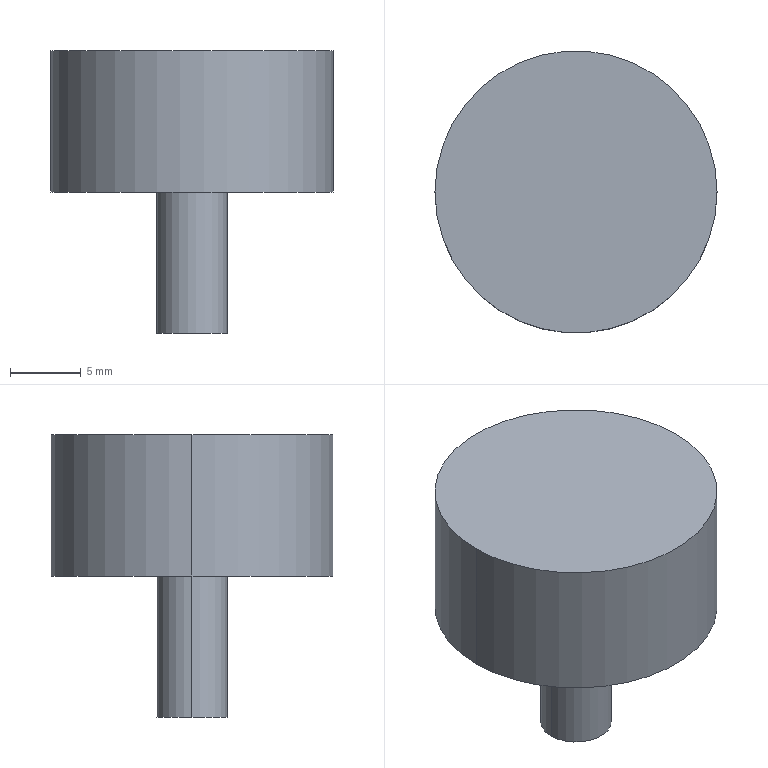Part | SolidWorks | features Extrusion 1, ICE 1 | 1 solid | 7 faces | box 20 x 20 x 20 mm | volume 3338 mm3 | cylinder 4 | plane 3 | commonest cylinder face diameters 5 x2 20 x2
STEP:
#1=CARTESIAN_POINT('',(10.,0.,20.));
#2=VERTEX_POINT('',#1);
#3=CARTESIAN_POINT('',(-10.,0.,20.));
#4=VERTEX_POINT('',#3);
#5=CARTESIAN_POINT('',(0.,0.,20.));
#6=DIRECTION('',(0.,0.,1.));
#7=DIRECTION('',(1.,0.,0.));
#8=AXIS2_PLACEMENT_3D('',#5,#6,#7);
#9=CIRCLE('',#8,10.);
#10=EDGE_CURVE('',#2,#4,#9,.T.);
#11=ORIENTED_EDGE('',*,*,#10,.F.);
#12=CARTESIAN_POINT('',(10.,0.,10.));
#13=VERTEX_POINT('',#12);
#14=CARTESIAN_POINT('',(10.,0.,20.));
#15=DIRECTION('',(0.,0.,-1.));
#16=VECTOR('',#15,1000.);
#17=LINE('',#14,#16);
#18=EDGE_CURVE('',#2,#13,#17,.T.);
#19=ORIENTED_EDGE('',*,*,#18,.T.);
#20=CARTESIAN_POINT('',(-10.,0.,10.));
#21=VERTEX_POINT('',#20);
#22=CARTESIAN_POINT('',(0.,0.,10.));
#23=DIRECTION('',(0.,0.,1.));
#24=DIRECTION('',(1.,0.,0.));
#25=AXIS2_PLACEMENT_3D('',#22,#23,#24);
#26=CIRCLE('',#25,10.);
#27=EDGE_CURVE('',#13,#21,#26,.T.);
#28=ORIENTED_EDGE('',*,*,#27,.T.);
#29=CARTESIAN_POINT('',(-10.,0.,20.));
#30=DIRECTION('',(0.,0.,-1.));
#31=VECTOR('',#30,1000.);
#32=LINE('',#29,#31);
#33=EDGE_CURVE('',#4,#21,#32,.T.);
#34=ORIENTED_EDGE('',*,*,#33,.F.);
#35=EDGE_LOOP('',(#11,#19,#28,#34));
#36=FACE_OUTER_BOUND('',#35,.T.);
#37=CARTESIAN_POINT('',(0.,0.,20.));
#38=DIRECTION('',(0.,0.,-1.));
#39=DIRECTION('',(-1.,0.,0.));
#40=AXIS2_PLACEMENT_3D('',#37,#38,#39);
#41=CYLINDRICAL_SURFACE('',#40,10.);
#42=ADVANCED_FACE('',(#36),#41,.T.);
#43=CARTESIAN_POINT('',(2.5,0.,10.));
#44=VERTEX_POINT('',#43);
#45=CARTESIAN_POINT('',(-2.5,0.,10.));
#46=VERTEX_POINT('',#45);
#47=CARTESIAN_POINT('',(0.,0.,10.));
#48=DIRECTION('',(0.,0.,1.));
#49=DIRECTION('',(1.,0.,0.));
#50=AXIS2_PLACEMENT_3D('',#47,#48,#49);
#51=CIRCLE('',#50,2.5);
#52=EDGE_CURVE('',#44,#46,#51,.T.);
#53=ORIENTED_EDGE('',*,*,#52,.F.);
#54=CARTESIAN_POINT('',(2.5,0.,0.));
#55=VERTEX_POINT('',#54);
#56=CARTESIAN_POINT('',(2.5,0.,10.));
#57=DIRECTION('',(0.,0.,-1.));
#58=VECTOR('',#57,1000.);
#59=LINE('',#56,#58);
#60=EDGE_CURVE('',#44,#55,#59,.T.);
#61=ORIENTED_EDGE('',*,*,#60,.T.);
#62=CARTESIAN_POINT('',(-2.5,0.,0.));
#63=VERTEX_POINT('',#62);
#64=CARTESIAN_POINT('',(0.,0.,0.));
#65=DIRECTION('',(0.,0.,1.));
#66=DIRECTION('',(1.,0.,0.));
#67=AXIS2_PLACEMENT_3D('',#64,#65,#66);
#68=CIRCLE('',#67,2.5);
#69=EDGE_CURVE('',#55,#63,#68,.T.);
#70=ORIENTED_EDGE('',*,*,#69,.T.);
#71=CARTESIAN_POINT('',(-2.5,0.,10.));
#72=DIRECTION('',(0.,0.,-1.));
#73=VECTOR('',#72,1000.);
#74=LINE('',#71,#73);
#75=EDGE_CURVE('',#46,#63,#74,.T.);
#76=ORIENTED_EDGE('',*,*,#75,.F.);
#77=EDGE_LOOP('',(#53,#61,#70,#76));
#78=FACE_OUTER_BOUND('',#77,.T.);
#79=CARTESIAN_POINT('',(0.,0.,10.));
#80=DIRECTION('',(0.,0.,-1.));
#81=DIRECTION('',(-1.,0.,0.));
#82=AXIS2_PLACEMENT_3D('',#79,#80,#81);
#83=CYLINDRICAL_SURFACE('',#82,2.5);
#84=ADVANCED_FACE('',(#78),#83,.T.);
#85=ORIENTED_EDGE('',*,*,#60,.F.);
#86=CARTESIAN_POINT('',(0.,0.,10.));
#87=DIRECTION('',(0.,0.,1.));
#88=DIRECTION('',(1.,0.,0.));
#89=AXIS2_PLACEMENT_3D('',#86,#87,#88);
#90=CIRCLE('',#89,2.5);
#91=EDGE_CURVE('',#46,#44,#90,.T.);
#92=ORIENTED_EDGE('',*,*,#91,.F.);
#93=ORIENTED_EDGE('',*,*,#75,.T.);
#94=CARTESIAN_POINT('',(0.,0.,0.));
#95=DIRECTION('',(0.,0.,1.));
#96=DIRECTION('',(1.,0.,0.));
#97=AXIS2_PLACEMENT_3D('',#94,#95,#96);
#98=CIRCLE('',#97,2.5);
#99=EDGE_CURVE('',#63,#55,#98,.T.);
#100=ORIENTED_EDGE('',*,*,#99,.T.);
#101=EDGE_LOOP('',(#85,#92,#93,#100));
#102=FACE_OUTER_BOUND('',#101,.T.);
#103=CARTESIAN_POINT('',(0.,0.,10.));
#104=DIRECTION('',(0.,0.,-1.));
#105=DIRECTION('',(-1.,0.,0.));
#106=AXIS2_PLACEMENT_3D('',#103,#104,#105);
#107=CYLINDRICAL_SURFACE('',#106,2.5);
#108=ADVANCED_FACE('',(#102),#107,.T.);
#109=ORIENTED_EDGE('',*,*,#99,.F.);
#110=ORIENTED_EDGE('',*,*,#69,.F.);
#111=EDGE_LOOP('',(#109,#110));
#112=FACE_OUTER_BOUND('',#111,.T.);
#113=CARTESIAN_POINT('',(0.,0.,0.));
#114=DIRECTION('',(0.,0.,1.));
#115=DIRECTION('',(1.,0.,0.));
#116=AXIS2_PLACEMENT_3D('',#113,#114,#115);
#117=PLANE('',#116);
#118=ADVANCED_FACE('',(#112),#117,.F.);
#119=ORIENTED_EDGE('',*,*,#18,.F.);
#120=CARTESIAN_POINT('',(0.,0.,20.));
#121=DIRECTION('',(0.,0.,1.));
#122=DIRECTION('',(1.,0.,0.));
#123=AXIS2_PLACEMENT_3D('',#120,#121,#122);
#124=CIRCLE('',#123,10.);
#125=EDGE_CURVE('',#4,#2,#124,.T.);
#126=ORIENTED_EDGE('',*,*,#125,.F.);
#127=ORIENTED_EDGE('',*,*,#33,.T.);
#128=CARTESIAN_POINT('',(0.,0.,10.));
#129=DIRECTION('',(0.,0.,1.));
#130=DIRECTION('',(1.,0.,0.));
#131=AXIS2_PLACEMENT_3D('',#128,#129,#130);
#132=CIRCLE('',#131,10.);
#133=EDGE_CURVE('',#21,#13,#132,.T.);
#134=ORIENTED_EDGE('',*,*,#133,.T.);
#135=EDGE_LOOP('',(#119,#126,#127,#134));
#136=FACE_OUTER_BOUND('',#135,.T.);
#137=CARTESIAN_POINT('',(0.,0.,20.));
#138=DIRECTION('',(0.,0.,-1.));
#139=DIRECTION('',(-1.,0.,0.));
#140=AXIS2_PLACEMENT_3D('',#137,#138,#139);
#141=CYLINDRICAL_SURFACE('',#140,10.);
#142=ADVANCED_FACE('',(#136),#141,.T.);
#143=ORIENTED_EDGE('',*,*,#125,.T.);
#144=ORIENTED_EDGE('',*,*,#10,.T.);
#145=EDGE_LOOP('',(#143,#144));
#146=FACE_OUTER_BOUND('',#145,.T.);
#147=CARTESIAN_POINT('',(0.,0.,20.));
#148=DIRECTION('',(0.,0.,1.));
#149=DIRECTION('',(1.,0.,0.));
#150=AXIS2_PLACEMENT_3D('',#147,#148,#149);
#151=PLANE('',#150);
#152=ADVANCED_FACE('',(#146),#151,.T.);
#153=ORIENTED_EDGE('',*,*,#91,.T.);
#154=ORIENTED_EDGE('',*,*,#52,.T.);
#155=EDGE_LOOP('',(#153,#154));
#156=FACE_BOUND('',#155,.T.);
#157=ORIENTED_EDGE('',*,*,#133,.F.);
#158=ORIENTED_EDGE('',*,*,#27,.F.);
#159=EDGE_LOOP('',(#157,#158));
#160=FACE_OUTER_BOUND('',#159,.T.);
#161=CARTESIAN_POINT('',(0.,0.,10.));
#162=DIRECTION('',(0.,0.,1.));
#163=DIRECTION('',(1.,0.,0.));
#164=AXIS2_PLACEMENT_3D('',#161,#162,#163);
#165=PLANE('',#164);
#166=ADVANCED_FACE('',(#156,#160),#165,.F.);
#167=CLOSED_SHELL('',(#42,#84,#108,#118,#142,#152,#166));
#168=MANIFOLD_SOLID_BREP('',#167);
#169=CARTESIAN_POINT('',(0.,0.,0.));
#170=DIRECTION('',(0.,0.,1.));
#171=DIRECTION('',(1.,0.,0.));
#172=AXIS2_PLACEMENT_3D('',#169,#170,#171);
#173=(LENGTH_UNIT()NAMED_UNIT(*)SI_UNIT(.MILLI.,.METRE.));
#174=UNCERTAINTY_MEASURE_WITH_UNIT(LENGTH_MEASURE(0.00001),#173,'','');
#175=(NAMED_UNIT(*)PLANE_ANGLE_UNIT()SI_UNIT($,.RADIAN.));
#176=(NAMED_UNIT(*)SI_UNIT($,.STERADIAN.)SOLID_ANGLE_UNIT());
#177=(GEOMETRIC_REPRESENTATION_CONTEXT(3)GLOBAL_UNCERTAINTY_ASSIGNED_CONTEXT((#174))GLOBAL_UNIT_ASSIGNED_CONTEXT((#173,#175,#176))REPRESENTATION_CONTEXT('',''));
#178=ADVANCED_BREP_SHAPE_REPRESENTATION('',(#168,#172),#177);